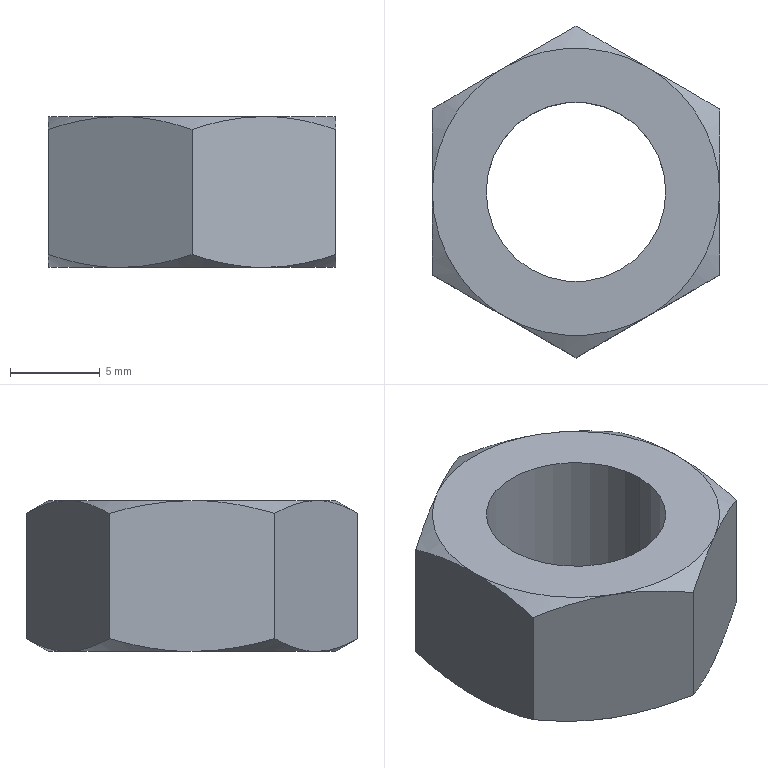Part | SolidWorks | features ICE 3, Extrusion 1, RefAxis 1 | 1 solid | 22 faces | box 16 x 18.475 x 8.4 mm | volume 1194 mm3 | cone 12 | plane 8 | cylinder 2 | commonest cylinder face diameters 10 x2
STEP:
#1=CARTESIAN_POINT('',(-5.,0.,0.));
#2=VERTEX_POINT('',#1);
#3=CARTESIAN_POINT('',(5.,0.,0.));
#4=VERTEX_POINT('',#3);
#5=CARTESIAN_POINT('',(0.,0.,0.));
#6=DIRECTION('',(0.,0.,1.));
#7=DIRECTION('',(1.,0.,0.));
#8=AXIS2_PLACEMENT_3D('',#5,#6,#7);
#9=CIRCLE('',#8,5.);
#10=EDGE_CURVE('',#2,#4,#9,.T.);
#11=ORIENTED_EDGE('',*,*,#10,.F.);
#12=CARTESIAN_POINT('',(-5.,0.,8.4));
#13=VERTEX_POINT('',#12);
#14=CARTESIAN_POINT('',(-5.,0.,0.));
#15=DIRECTION('',(0.,0.,1.));
#16=VECTOR('',#15,1000.);
#17=LINE('',#14,#16);
#18=EDGE_CURVE('',#2,#13,#17,.T.);
#19=ORIENTED_EDGE('',*,*,#18,.T.);
#20=CARTESIAN_POINT('',(5.,0.,8.4));
#21=VERTEX_POINT('',#20);
#22=CARTESIAN_POINT('',(0.,0.,8.4));
#23=DIRECTION('',(0.,0.,1.));
#24=DIRECTION('',(1.,0.,0.));
#25=AXIS2_PLACEMENT_3D('',#22,#23,#24);
#26=CIRCLE('',#25,5.);
#27=EDGE_CURVE('',#13,#21,#26,.T.);
#28=ORIENTED_EDGE('',*,*,#27,.T.);
#29=CARTESIAN_POINT('',(5.,0.,0.));
#30=DIRECTION('',(0.,0.,1.));
#31=VECTOR('',#30,1000.);
#32=LINE('',#29,#31);
#33=EDGE_CURVE('',#4,#21,#32,.T.);
#34=ORIENTED_EDGE('',*,*,#33,.F.);
#35=EDGE_LOOP('',(#11,#19,#28,#34));
#36=FACE_OUTER_BOUND('',#35,.T.);
#37=CARTESIAN_POINT('',(0.,0.,0.));
#38=DIRECTION('',(0.,0.,1.));
#39=DIRECTION('',(1.,0.,0.));
#40=AXIS2_PLACEMENT_3D('',#37,#38,#39);
#41=CYLINDRICAL_SURFACE('',#40,5.);
#42=ADVANCED_FACE('',(#36),#41,.F.);
#43=CARTESIAN_POINT('',(0.,9.238,0.7145));
#44=VERTEX_POINT('',#43);
#45=CARTESIAN_POINT('',(4.,6.928,0.));
#46=VERTEX_POINT('',#45);
#47=CARTESIAN_POINT('',(0.,9.238,0.7145));
#48=CARTESIAN_POINT('',(0.6543,8.86,0.4964));
#49=CARTESIAN_POINT('',(1.313,8.479,0.3167));
#50=CARTESIAN_POINT('',(2.646,7.71,0.0681));
#51=CARTESIAN_POINT('',(3.319,7.322,0.));
#52=CARTESIAN_POINT('',(4.,6.928,0.));
#53=B_SPLINE_CURVE_WITH_KNOTS('',3,(#47,#48,#49,#50,#51,#52),.UNSPECIFIED.,.F.,.F.,(4,2,4),(0.000000238,0.002337,0.004674),.UNSPECIFIED.);
#54=EDGE_CURVE('',#44,#46,#53,.T.);
#55=ORIENTED_EDGE('',*,*,#54,.F.);
#56=CARTESIAN_POINT('',(0.,9.238,7.685));
#57=VERTEX_POINT('',#56);
#58=CARTESIAN_POINT('',(0.,9.238,8.4));
#59=DIRECTION('',(0.,0.,-1.));
#60=VECTOR('',#59,1000.);
#61=LINE('',#58,#60);
#62=EDGE_CURVE('',#57,#44,#61,.T.);
#63=ORIENTED_EDGE('',*,*,#62,.F.);
#64=CARTESIAN_POINT('',(4.,6.928,8.4));
#65=VERTEX_POINT('',#64);
#66=CARTESIAN_POINT('',(4.,6.928,8.4));
#67=CARTESIAN_POINT('',(3.661,7.124,8.4));
#68=CARTESIAN_POINT('',(3.32,7.321,8.383));
#69=CARTESIAN_POINT('',(2.645,7.711,8.318));
#70=CARTESIAN_POINT('',(2.31,7.904,8.269));
#71=CARTESIAN_POINT('',(1.311,8.481,8.083));
#72=CARTESIAN_POINT('',(0.6527,8.861,7.903));
#73=CARTESIAN_POINT('',(0.,9.238,7.685));
#74=B_SPLINE_CURVE_WITH_KNOTS('',3,(#66,#67,#68,#69,#70,#71,#72,#73),.UNSPECIFIED.,.F.,.F.,(4,2,2,4),(0.004674,0.005838,0.007002,0.00933),.UNSPECIFIED.);
#75=EDGE_CURVE('',#65,#57,#74,.T.);
#76=ORIENTED_EDGE('',*,*,#75,.F.);
#77=CARTESIAN_POINT('',(8.,4.619,7.685));
#78=VERTEX_POINT('',#77);
#79=CARTESIAN_POINT('',(8.,4.619,7.685));
#80=CARTESIAN_POINT('',(7.346,4.997,7.904));
#81=CARTESIAN_POINT('',(6.687,5.377,8.083));
#82=CARTESIAN_POINT('',(5.354,6.146,8.332));
#83=CARTESIAN_POINT('',(4.681,6.535,8.4));
#84=CARTESIAN_POINT('',(4.,6.928,8.4));
#85=B_SPLINE_CURVE_WITH_KNOTS('',3,(#79,#80,#81,#82,#83,#84),.UNSPECIFIED.,.F.,.F.,(4,2,4),(0.000000238,0.002337,0.004674),.UNSPECIFIED.);
#86=EDGE_CURVE('',#78,#65,#85,.T.);
#87=ORIENTED_EDGE('',*,*,#86,.F.);
#88=CARTESIAN_POINT('',(8.,4.619,0.7145));
#89=VERTEX_POINT('',#88);
#90=CARTESIAN_POINT('',(8.,4.619,8.4));
#91=DIRECTION('',(0.,0.,-1.));
#92=VECTOR('',#91,1000.);
#93=LINE('',#90,#92);
#94=EDGE_CURVE('',#78,#89,#93,.T.);
#95=ORIENTED_EDGE('',*,*,#94,.T.);
#96=CARTESIAN_POINT('',(4.,6.928,0.));
#97=CARTESIAN_POINT('',(4.339,6.732,0.));
#98=CARTESIAN_POINT('',(4.68,6.535,0.01689));
#99=CARTESIAN_POINT('',(5.355,6.146,0.08225));
#100=CARTESIAN_POINT('',(5.69,5.952,0.1307));
#101=CARTESIAN_POINT('',(6.689,5.376,0.3174));
#102=CARTESIAN_POINT('',(7.347,4.996,0.497));
#103=CARTESIAN_POINT('',(8.,4.619,0.7145));
#104=B_SPLINE_CURVE_WITH_KNOTS('',3,(#96,#97,#98,#99,#100,#101,#102,#103),.UNSPECIFIED.,.F.,.F.,(4,2,2,4),(0.004674,0.005838,0.007002,0.00933),.UNSPECIFIED.);
#105=EDGE_CURVE('',#46,#89,#104,.T.);
#106=ORIENTED_EDGE('',*,*,#105,.F.);
#107=EDGE_LOOP('',(#55,#63,#76,#87,#95,#106));
#108=FACE_OUTER_BOUND('',#107,.T.);
#109=CARTESIAN_POINT('',(8.,4.619,8.4));
#110=DIRECTION('',(-0.5,-0.866,0.));
#111=DIRECTION('',(0.866,-0.5,0.));
#112=AXIS2_PLACEMENT_3D('',#109,#110,#111);
#113=PLANE('',#112);
#114=ADVANCED_FACE('',(#108),#113,.F.);
#115=CARTESIAN_POINT('',(-8.,4.619,0.7145));
#116=VERTEX_POINT('',#115);
#117=CARTESIAN_POINT('',(-4.,6.928,0.));
#118=VERTEX_POINT('',#117);
#119=CARTESIAN_POINT('',(-8.,4.619,0.7145));
#120=CARTESIAN_POINT('',(-7.346,4.997,0.4964));
#121=CARTESIAN_POINT('',(-6.687,5.377,0.3167));
#122=CARTESIAN_POINT('',(-5.354,6.146,0.0681));
#123=CARTESIAN_POINT('',(-4.681,6.535,0.));
#124=CARTESIAN_POINT('',(-4.,6.928,0.));
#125=B_SPLINE_CURVE_WITH_KNOTS('',3,(#119,#120,#121,#122,#123,#124),.UNSPECIFIED.,.F.,.F.,(4,2,4),(0.000000238,0.002337,0.004674),.UNSPECIFIED.);
#126=EDGE_CURVE('',#116,#118,#125,.T.);
#127=ORIENTED_EDGE('',*,*,#126,.F.);
#128=CARTESIAN_POINT('',(-8.,4.619,7.685));
#129=VERTEX_POINT('',#128);
#130=CARTESIAN_POINT('',(-8.,4.619,8.4));
#131=DIRECTION('',(0.,0.,-1.));
#132=VECTOR('',#131,1000.);
#133=LINE('',#130,#132);
#134=EDGE_CURVE('',#129,#116,#133,.T.);
#135=ORIENTED_EDGE('',*,*,#134,.F.);
#136=CARTESIAN_POINT('',(-4.,6.928,8.4));
#137=VERTEX_POINT('',#136);
#138=CARTESIAN_POINT('',(-4.,6.928,8.4));
#139=CARTESIAN_POINT('',(-4.339,6.732,8.4));
#140=CARTESIAN_POINT('',(-4.68,6.535,8.383));
#141=CARTESIAN_POINT('',(-5.355,6.146,8.318));
#142=CARTESIAN_POINT('',(-5.69,5.952,8.269));
#143=CARTESIAN_POINT('',(-6.689,5.376,8.083));
#144=CARTESIAN_POINT('',(-7.347,4.996,7.903));
#145=CARTESIAN_POINT('',(-8.,4.619,7.685));
#146=B_SPLINE_CURVE_WITH_KNOTS('',3,(#138,#139,#140,#141,#142,#143,#144,#145),.UNSPECIFIED.,.F.,.F.,(4,2,2,4),(0.004674,0.005838,0.007002,0.00933),.UNSPECIFIED.);
#147=EDGE_CURVE('',#137,#129,#146,.T.);
#148=ORIENTED_EDGE('',*,*,#147,.F.);
#149=CARTESIAN_POINT('',(0.,9.238,7.685));
#150=CARTESIAN_POINT('',(-0.6543,8.86,7.904));
#151=CARTESIAN_POINT('',(-1.313,8.479,8.083));
#152=CARTESIAN_POINT('',(-2.646,7.71,8.332));
#153=CARTESIAN_POINT('',(-3.319,7.322,8.4));
#154=CARTESIAN_POINT('',(-4.,6.928,8.4));
#155=B_SPLINE_CURVE_WITH_KNOTS('',3,(#149,#150,#151,#152,#153,#154),.UNSPECIFIED.,.F.,.F.,(4,2,4),(0.000000238,0.002337,0.004674),.UNSPECIFIED.);
#156=EDGE_CURVE('',#57,#137,#155,.T.);
#157=ORIENTED_EDGE('',*,*,#156,.F.);
#158=ORIENTED_EDGE('',*,*,#62,.T.);
#159=CARTESIAN_POINT('',(-4.,6.928,0.));
#160=CARTESIAN_POINT('',(-3.661,7.124,0.));
#161=CARTESIAN_POINT('',(-3.32,7.321,0.01689));
#162=CARTESIAN_POINT('',(-2.645,7.711,0.08225));
#163=CARTESIAN_POINT('',(-2.31,7.904,0.1307));
#164=CARTESIAN_POINT('',(-1.311,8.481,0.3174));
#165=CARTESIAN_POINT('',(-0.6527,8.861,0.497));
#166=CARTESIAN_POINT('',(0.,9.238,0.7145));
#167=B_SPLINE_CURVE_WITH_KNOTS('',3,(#159,#160,#161,#162,#163,#164,#165,#166),.UNSPECIFIED.,.F.,.F.,(4,2,2,4),(0.004674,0.005838,0.007002,0.00933),.UNSPECIFIED.);
#168=EDGE_CURVE('',#118,#44,#167,.T.);
#169=ORIENTED_EDGE('',*,*,#168,.F.);
#170=EDGE_LOOP('',(#127,#135,#148,#157,#158,#169));
#171=FACE_OUTER_BOUND('',#170,.T.);
#172=CARTESIAN_POINT('',(0.,9.238,8.4));
#173=DIRECTION('',(0.5,-0.866,0.));
#174=DIRECTION('',(0.866,0.5,0.));
#175=AXIS2_PLACEMENT_3D('',#172,#173,#174);
#176=PLANE('',#175);
#177=ADVANCED_FACE('',(#171),#176,.F.);
#178=CARTESIAN_POINT('',(-8.,-4.619,0.7145));
#179=VERTEX_POINT('',#178);
#180=CARTESIAN_POINT('',(-8.,0.,0.));
#181=VERTEX_POINT('',#180);
#182=CARTESIAN_POINT('',(-8.,-4.619,0.7145));
#183=CARTESIAN_POINT('',(-8.,-3.867,0.4975));
#184=CARTESIAN_POINT('',(-8.,-3.098,0.3157));
#185=CARTESIAN_POINT('',(-8.,-1.557,0.06719));
#186=CARTESIAN_POINT('',(-8.,-0.7811,0.));
#187=CARTESIAN_POINT('',(-8.,0.,0.));
#188=B_SPLINE_CURVE_WITH_KNOTS('',3,(#182,#183,#184,#185,#186,#187),.UNSPECIFIED.,.F.,.F.,(4,2,4),(0.008455,0.01079,0.01313),.UNSPECIFIED.);
#189=EDGE_CURVE('',#179,#181,#188,.T.);
#190=ORIENTED_EDGE('',*,*,#189,.F.);
#191=CARTESIAN_POINT('',(-8.,-4.619,7.685));
#192=VERTEX_POINT('',#191);
#193=CARTESIAN_POINT('',(-8.,-4.619,8.4));
#194=DIRECTION('',(0.,0.,-1.));
#195=VECTOR('',#194,1000.);
#196=LINE('',#193,#195);
#197=EDGE_CURVE('',#192,#179,#196,.T.);
#198=ORIENTED_EDGE('',*,*,#197,.F.);
#199=CARTESIAN_POINT('',(-8.,0.,8.4));
#200=VERTEX_POINT('',#199);
#201=CARTESIAN_POINT('',(-8.,0.,8.4));
#202=CARTESIAN_POINT('',(-8.,-0.7811,8.4));
#203=CARTESIAN_POINT('',(-8.,-1.557,8.333));
#204=CARTESIAN_POINT('',(-8.,-3.098,8.084));
#205=CARTESIAN_POINT('',(-8.,-3.867,7.903));
#206=CARTESIAN_POINT('',(-8.,-4.619,7.685));
#207=B_SPLINE_CURVE_WITH_KNOTS('',3,(#201,#202,#203,#204,#205,#206),.UNSPECIFIED.,.F.,.F.,(4,2,4),(0.03088,0.03322,0.03555),.UNSPECIFIED.);
#208=EDGE_CURVE('',#200,#192,#207,.T.);
#209=ORIENTED_EDGE('',*,*,#208,.F.);
#210=CARTESIAN_POINT('',(-8.,4.619,7.685));
#211=CARTESIAN_POINT('',(-8.,3.872,7.901));
#212=CARTESIAN_POINT('',(-8.,3.115,8.081));
#213=CARTESIAN_POINT('',(-8.,1.574,8.331));
#214=CARTESIAN_POINT('',(-8.,0.7817,8.4));
#215=CARTESIAN_POINT('',(-8.,0.,8.4));
#216=B_SPLINE_CURVE_WITH_KNOTS('',3,(#210,#211,#212,#213,#214,#215),.UNSPECIFIED.,.F.,.F.,(4,2,4),(0.0262,0.02854,0.03088),.UNSPECIFIED.);
#217=EDGE_CURVE('',#129,#200,#216,.T.);
#218=ORIENTED_EDGE('',*,*,#217,.F.);
#219=ORIENTED_EDGE('',*,*,#134,.T.);
#220=CARTESIAN_POINT('',(-8.,0.,0.));
#221=CARTESIAN_POINT('',(-8.,0.7817,0.));
#222=CARTESIAN_POINT('',(-8.,1.574,0.06908));
#223=CARTESIAN_POINT('',(-8.,3.115,0.3194));
#224=CARTESIAN_POINT('',(-8.,3.872,0.4989));
#225=CARTESIAN_POINT('',(-8.,4.619,0.7145));
#226=B_SPLINE_CURVE_WITH_KNOTS('',3,(#220,#221,#222,#223,#224,#225),.UNSPECIFIED.,.F.,.F.,(4,2,4),(0.01313,0.01547,0.01781),.UNSPECIFIED.);
#227=EDGE_CURVE('',#181,#116,#226,.T.);
#228=ORIENTED_EDGE('',*,*,#227,.F.);
#229=EDGE_LOOP('',(#190,#198,#209,#218,#219,#228));
#230=FACE_OUTER_BOUND('',#229,.T.);
#231=CARTESIAN_POINT('',(-8.,4.619,8.4));
#232=DIRECTION('',(1.,0.,0.));
#233=DIRECTION('',(0.,0.,-1.));
#234=AXIS2_PLACEMENT_3D('',#231,#232,#233);
#235=PLANE('',#234);
#236=ADVANCED_FACE('',(#230),#235,.F.);
#237=CARTESIAN_POINT('',(0.,-9.238,0.7145));
#238=VERTEX_POINT('',#237);
#239=CARTESIAN_POINT('',(-4.,-6.928,0.));
#240=VERTEX_POINT('',#239);
#241=CARTESIAN_POINT('',(0.,-9.238,0.7145));
#242=CARTESIAN_POINT('',(-0.6543,-8.86,0.4964));
#243=CARTESIAN_POINT('',(-1.313,-8.479,0.3167));
#244=CARTESIAN_POINT('',(-2.646,-7.71,0.0681));
#245=CARTESIAN_POINT('',(-3.319,-7.322,0.));
#246=CARTESIAN_POINT('',(-4.,-6.928,0.));
#247=B_SPLINE_CURVE_WITH_KNOTS('',3,(#241,#242,#243,#244,#245,#246),.UNSPECIFIED.,.F.,.F.,(4,2,4),(0.000000238,0.002337,0.004674),.UNSPECIFIED.);
#248=EDGE_CURVE('',#238,#240,#247,.T.);
#249=ORIENTED_EDGE('',*,*,#248,.F.);
#250=CARTESIAN_POINT('',(0.,-9.238,7.685));
#251=VERTEX_POINT('',#250);
#252=CARTESIAN_POINT('',(0.,-9.238,8.4));
#253=DIRECTION('',(0.,0.,-1.));
#254=VECTOR('',#253,1000.);
#255=LINE('',#252,#254);
#256=EDGE_CURVE('',#251,#238,#255,.T.);
#257=ORIENTED_EDGE('',*,*,#256,.F.);
#258=CARTESIAN_POINT('',(-4.,-6.928,8.4));
#259=VERTEX_POINT('',#258);
#260=CARTESIAN_POINT('',(-4.,-6.928,8.4));
#261=CARTESIAN_POINT('',(-3.661,-7.124,8.4));
#262=CARTESIAN_POINT('',(-3.32,-7.321,8.383));
#263=CARTESIAN_POINT('',(-2.645,-7.711,8.318));
#264=CARTESIAN_POINT('',(-2.31,-7.904,8.269));
#265=CARTESIAN_POINT('',(-1.311,-8.481,8.083));
#266=CARTESIAN_POINT('',(-0.6527,-8.861,7.903));
#267=CARTESIAN_POINT('',(0.,-9.238,7.685));
#268=B_SPLINE_CURVE_WITH_KNOTS('',3,(#260,#261,#262,#263,#264,#265,#266,#267),.UNSPECIFIED.,.F.,.F.,(4,2,2,4),(0.004674,0.005838,0.007002,0.00933),.UNSPECIFIED.);
#269=EDGE_CURVE('',#259,#251,#268,.T.);
#270=ORIENTED_EDGE('',*,*,#269,.F.);
#271=CARTESIAN_POINT('',(-8.,-4.619,7.685));
#272=CARTESIAN_POINT('',(-7.346,-4.997,7.904));
#273=CARTESIAN_POINT('',(-6.687,-5.377,8.083));
#274=CARTESIAN_POINT('',(-5.354,-6.146,8.332));
#275=CARTESIAN_POINT('',(-4.681,-6.535,8.4));
#276=CARTESIAN_POINT('',(-4.,-6.928,8.4));
#277=B_SPLINE_CURVE_WITH_KNOTS('',3,(#271,#272,#273,#274,#275,#276),.UNSPECIFIED.,.F.,.F.,(4,2,4),(0.000000238,0.002337,0.004674),.UNSPECIFIED.);
#278=EDGE_CURVE('',#192,#259,#277,.T.);
#279=ORIENTED_EDGE('',*,*,#278,.F.);
#280=ORIENTED_EDGE('',*,*,#197,.T.);
#281=CARTESIAN_POINT('',(-4.,-6.928,0.));
#282=CARTESIAN_POINT('',(-4.339,-6.732,0.));
#283=CARTESIAN_POINT('',(-4.68,-6.535,0.01689));
#284=CARTESIAN_POINT('',(-5.355,-6.146,0.08225));
#285=CARTESIAN_POINT('',(-5.69,-5.952,0.1307));
#286=CARTESIAN_POINT('',(-6.689,-5.376,0.3174));
#287=CARTESIAN_POINT('',(-7.347,-4.996,0.497));
#288=CARTESIAN_POINT('',(-8.,-4.619,0.7145));
#289=B_SPLINE_CURVE_WITH_KNOTS('',3,(#281,#282,#283,#284,#285,#286,#287,#288),.UNSPECIFIED.,.F.,.F.,(4,2,2,4),(0.004674,0.005838,0.007002,0.00933),.UNSPECIFIED.);
#290=EDGE_CURVE('',#240,#179,#289,.T.);
#291=ORIENTED_EDGE('',*,*,#290,.F.);
#292=EDGE_LOOP('',(#249,#257,#270,#279,#280,#291));
#293=FACE_OUTER_BOUND('',#292,.T.);
#294=CARTESIAN_POINT('',(-8.,-4.619,8.4));
#295=DIRECTION('',(0.5,0.866,0.));
#296=DIRECTION('',(-0.866,0.5,0.));
#297=AXIS2_PLACEMENT_3D('',#294,#295,#296);
#298=PLANE('',#297);
#299=ADVANCED_FACE('',(#293),#298,.F.);
#300=CARTESIAN_POINT('',(8.,-4.619,0.7145));
#301=VERTEX_POINT('',#300);
#302=CARTESIAN_POINT('',(4.,-6.928,0.));
#303=VERTEX_POINT('',#302);
#304=CARTESIAN_POINT('',(8.,-4.619,0.7145));
#305=CARTESIAN_POINT('',(7.346,-4.997,0.4964));
#306=CARTESIAN_POINT('',(6.687,-5.377,0.3167));
#307=CARTESIAN_POINT('',(5.354,-6.146,0.0681));
#308=CARTESIAN_POINT('',(4.681,-6.535,0.));
#309=CARTESIAN_POINT('',(4.,-6.928,0.));
#310=B_SPLINE_CURVE_WITH_KNOTS('',3,(#304,#305,#306,#307,#308,#309),.UNSPECIFIED.,.F.,.F.,(4,2,4),(0.000000238,0.002337,0.004674),.UNSPECIFIED.);
#311=EDGE_CURVE('',#301,#303,#310,.T.);
#312=ORIENTED_EDGE('',*,*,#311,.F.);
#313=CARTESIAN_POINT('',(8.,-4.619,7.685));
#314=VERTEX_POINT('',#313);
#315=CARTESIAN_POINT('',(8.,-4.619,8.4));
#316=DIRECTION('',(0.,0.,-1.));
#317=VECTOR('',#316,1000.);
#318=LINE('',#315,#317);
#319=EDGE_CURVE('',#314,#301,#318,.T.);
#320=ORIENTED_EDGE('',*,*,#319,.F.);
#321=CARTESIAN_POINT('',(4.,-6.928,8.4));
#322=VERTEX_POINT('',#321);
#323=CARTESIAN_POINT('',(4.,-6.928,8.4));
#324=CARTESIAN_POINT('',(4.339,-6.732,8.4));
#325=CARTESIAN_POINT('',(4.68,-6.535,8.383));
#326=CARTESIAN_POINT('',(5.355,-6.146,8.318));
#327=CARTESIAN_POINT('',(5.69,-5.952,8.269));
#328=CARTESIAN_POINT('',(6.689,-5.376,8.083));
#329=CARTESIAN_POINT('',(7.347,-4.996,7.903));
#330=CARTESIAN_POINT('',(8.,-4.619,7.685));
#331=B_SPLINE_CURVE_WITH_KNOTS('',3,(#323,#324,#325,#326,#327,#328,#329,#330),.UNSPECIFIED.,.F.,.F.,(4,2,2,4),(0.004674,0.005838,0.007002,0.00933),.UNSPECIFIED.);
#332=EDGE_CURVE('',#322,#314,#331,.T.);
#333=ORIENTED_EDGE('',*,*,#332,.F.);
#334=CARTESIAN_POINT('',(0.,-9.238,7.685));
#335=CARTESIAN_POINT('',(0.6543,-8.86,7.904));
#336=CARTESIAN_POINT('',(1.313,-8.479,8.083));
#337=CARTESIAN_POINT('',(2.646,-7.71,8.332));
#338=CARTESIAN_POINT('',(3.319,-7.322,8.4));
#339=CARTESIAN_POINT('',(4.,-6.928,8.4));
#340=B_SPLINE_CURVE_WITH_KNOTS('',3,(#334,#335,#336,#337,#338,#339),.UNSPECIFIED.,.F.,.F.,(4,2,4),(0.000000238,0.002337,0.004674),.UNSPECIFIED.);
#341=EDGE_CURVE('',#251,#322,#340,.T.);
#342=ORIENTED_EDGE('',*,*,#341,.F.);
#343=ORIENTED_EDGE('',*,*,#256,.T.);
#344=CARTESIAN_POINT('',(4.,-6.928,0.));
#345=CARTESIAN_POINT('',(3.661,-7.124,0.));
#346=CARTESIAN_POINT('',(3.32,-7.321,0.01689));
#347=CARTESIAN_POINT('',(2.645,-7.711,0.08225));
#348=CARTESIAN_POINT('',(2.31,-7.904,0.1307));
#349=CARTESIAN_POINT('',(1.311,-8.481,0.3174));
#350=CARTESIAN_POINT('',(0.6527,-8.861,0.497));
#351=CARTESIAN_POINT('',(0.,-9.238,0.7145));
#352=B_SPLINE_CURVE_WITH_KNOTS('',3,(#344,#345,#346,#347,#348,#349,#350,#351),.UNSPECIFIED.,.F.,.F.,(4,2,2,4),(0.004674,0.005838,0.007002,0.00933),.UNSPECIFIED.);
#353=EDGE_CURVE('',#303,#238,#352,.T.);
#354=ORIENTED_EDGE('',*,*,#353,.F.);
#355=EDGE_LOOP('',(#312,#320,#333,#342,#343,#354));
#356=FACE_OUTER_BOUND('',#355,.T.);
#357=CARTESIAN_POINT('',(0.,-9.238,8.4));
#358=DIRECTION('',(-0.5,0.866,0.));
#359=DIRECTION('',(-0.866,-0.5,0.));
#360=AXIS2_PLACEMENT_3D('',#357,#358,#359);
#361=PLANE('',#360);
#362=ADVANCED_FACE('',(#356),#361,.F.);
#363=CARTESIAN_POINT('',(8.,0.,0.));
#364=VERTEX_POINT('',#363);
#365=CARTESIAN_POINT('',(8.,4.619,0.7145));
#366=CARTESIAN_POINT('',(8.,3.872,0.4989));
#367=CARTESIAN_POINT('',(8.,3.115,0.3194));
#368=CARTESIAN_POINT('',(8.,1.574,0.06908));
#369=CARTESIAN_POINT('',(8.,0.7817,0.));
#370=CARTESIAN_POINT('',(8.,0.,0.));
#371=B_SPLINE_CURVE_WITH_KNOTS('',3,(#365,#366,#367,#368,#369,#370),.UNSPECIFIED.,.F.,.F.,(4,2,4),(0.0262,0.02854,0.03088),.UNSPECIFIED.);
#372=EDGE_CURVE('',#89,#364,#371,.T.);
#373=ORIENTED_EDGE('',*,*,#372,.F.);
#374=ORIENTED_EDGE('',*,*,#94,.F.);
#375=CARTESIAN_POINT('',(8.,0.,8.4));
#376=VERTEX_POINT('',#375);
#377=CARTESIAN_POINT('',(8.,0.,8.4));
#378=CARTESIAN_POINT('',(8.,0.7817,8.4));
#379=CARTESIAN_POINT('',(8.,1.574,8.331));
#380=CARTESIAN_POINT('',(8.,3.115,8.081));
#381=CARTESIAN_POINT('',(8.,3.872,7.901));
#382=CARTESIAN_POINT('',(8.,4.619,7.685));
#383=B_SPLINE_CURVE_WITH_KNOTS('',3,(#377,#378,#379,#380,#381,#382),.UNSPECIFIED.,.F.,.F.,(4,2,4),(0.01313,0.01547,0.01781),.UNSPECIFIED.);
#384=EDGE_CURVE('',#376,#78,#383,.T.);
#385=ORIENTED_EDGE('',*,*,#384,.F.);
#386=CARTESIAN_POINT('',(8.,-4.619,7.685));
#387=CARTESIAN_POINT('',(8.,-3.867,7.903));
#388=CARTESIAN_POINT('',(8.,-3.098,8.084));
#389=CARTESIAN_POINT('',(8.,-1.557,8.333));
#390=CARTESIAN_POINT('',(8.,-0.7811,8.4));
#391=CARTESIAN_POINT('',(8.,0.,8.4));
#392=B_SPLINE_CURVE_WITH_KNOTS('',3,(#386,#387,#388,#389,#390,#391),.UNSPECIFIED.,.F.,.F.,(4,2,4),(0.008455,0.01079,0.01313),.UNSPECIFIED.);
#393=EDGE_CURVE('',#314,#376,#392,.T.);
#394=ORIENTED_EDGE('',*,*,#393,.F.);
#395=ORIENTED_EDGE('',*,*,#319,.T.);
#396=CARTESIAN_POINT('',(8.,0.,0.));
#397=CARTESIAN_POINT('',(8.,-0.7811,0.));
#398=CARTESIAN_POINT('',(8.,-1.557,0.06719));
#399=CARTESIAN_POINT('',(8.,-3.098,0.3157));
#400=CARTESIAN_POINT('',(8.,-3.867,0.4975));
#401=CARTESIAN_POINT('',(8.,-4.619,0.7145));
#402=B_SPLINE_CURVE_WITH_KNOTS('',3,(#396,#397,#398,#399,#400,#401),.UNSPECIFIED.,.F.,.F.,(4,2,4),(0.03088,0.03322,0.03555),.UNSPECIFIED.);
#403=EDGE_CURVE('',#364,#301,#402,.T.);
#404=ORIENTED_EDGE('',*,*,#403,.F.);
#405=EDGE_LOOP('',(#373,#374,#385,#394,#395,#404));
#406=FACE_OUTER_BOUND('',#405,.T.);
#407=CARTESIAN_POINT('',(8.,-4.619,8.4));
#408=DIRECTION('',(-1.,0.,0.));
#409=DIRECTION('',(0.,-1.,0.));
#410=AXIS2_PLACEMENT_3D('',#407,#408,#409);
#411=PLANE('',#410);
#412=ADVANCED_FACE('',(#406),#411,.F.);
#413=CARTESIAN_POINT('',(0.,0.,0.));
#414=DIRECTION('',(0.,0.,1.));
#415=DIRECTION('',(1.,0.,0.));
#416=AXIS2_PLACEMENT_3D('',#413,#414,#415);
#417=CIRCLE('',#416,5.);
#418=EDGE_CURVE('',#4,#2,#417,.T.);
#419=ORIENTED_EDGE('',*,*,#418,.T.);
#420=ORIENTED_EDGE('',*,*,#10,.T.);
#421=EDGE_LOOP('',(#419,#420));
#422=FACE_BOUND('',#421,.T.);
#423=CARTESIAN_POINT('',(0.,0.,0.));
#424=DIRECTION('',(0.,0.,1.));
#425=DIRECTION('',(1.,0.,0.));
#426=AXIS2_PLACEMENT_3D('',#423,#424,#425);
#427=CIRCLE('',#426,8.);
#428=EDGE_CURVE('',#364,#46,#427,.T.);
#429=ORIENTED_EDGE('',*,*,#428,.F.);
#430=CARTESIAN_POINT('',(0.,0.,0.));
#431=DIRECTION('',(0.,0.,1.));
#432=DIRECTION('',(1.,0.,0.));
#433=AXIS2_PLACEMENT_3D('',#430,#431,#432);
#434=CIRCLE('',#433,8.);
#435=EDGE_CURVE('',#303,#364,#434,.T.);
#436=ORIENTED_EDGE('',*,*,#435,.F.);
#437=CARTESIAN_POINT('',(0.,0.,0.));
#438=DIRECTION('',(0.,0.,1.));
#439=DIRECTION('',(1.,0.,0.));
#440=AXIS2_PLACEMENT_3D('',#437,#438,#439);
#441=CIRCLE('',#440,8.);
#442=EDGE_CURVE('',#240,#303,#441,.T.);
#443=ORIENTED_EDGE('',*,*,#442,.F.);
#444=CARTESIAN_POINT('',(0.,0.,0.));
#445=DIRECTION('',(0.,0.,1.));
#446=DIRECTION('',(1.,0.,0.));
#447=AXIS2_PLACEMENT_3D('',#444,#445,#446);
#448=CIRCLE('',#447,8.);
#449=EDGE_CURVE('',#181,#240,#448,.T.);
#450=ORIENTED_EDGE('',*,*,#449,.F.);
#451=CARTESIAN_POINT('',(0.,0.,0.));
#452=DIRECTION('',(0.,0.,-1.));
#453=DIRECTION('',(-1.,0.,0.));
#454=AXIS2_PLACEMENT_3D('',#451,#452,#453);
#455=CIRCLE('',#454,8.);
#456=EDGE_CURVE('',#181,#118,#455,.T.);
#457=ORIENTED_EDGE('',*,*,#456,.T.);
#458=CARTESIAN_POINT('',(0.,0.,0.));
#459=DIRECTION('',(0.,0.,1.));
#460=DIRECTION('',(1.,0.,0.));
#461=AXIS2_PLACEMENT_3D('',#458,#459,#460);
#462=CIRCLE('',#461,8.);
#463=EDGE_CURVE('',#46,#118,#462,.T.);
#464=ORIENTED_EDGE('',*,*,#463,.F.);
#465=EDGE_LOOP('',(#429,#436,#443,#450,#457,#464));
#466=FACE_OUTER_BOUND('',#465,.T.);
#467=CARTESIAN_POINT('',(0.,0.,0.));
#468=DIRECTION('',(0.,0.,1.));
#469=DIRECTION('',(1.,0.,0.));
#470=AXIS2_PLACEMENT_3D('',#467,#468,#469);
#471=PLANE('',#470);
#472=ADVANCED_FACE('',(#422,#466),#471,.F.);
#473=CARTESIAN_POINT('',(0.,0.,8.4));
#474=DIRECTION('',(0.,0.,1.));
#475=DIRECTION('',(1.,0.,0.));
#476=AXIS2_PLACEMENT_3D('',#473,#474,#475);
#477=CIRCLE('',#476,5.);
#478=EDGE_CURVE('',#21,#13,#477,.T.);
#479=ORIENTED_EDGE('',*,*,#478,.F.);
#480=ORIENTED_EDGE('',*,*,#27,.F.);
#481=EDGE_LOOP('',(#479,#480));
#482=FACE_BOUND('',#481,.T.);
#483=CARTESIAN_POINT('',(0.,0.,8.4));
#484=DIRECTION('',(0.,0.,1.));
#485=DIRECTION('',(1.,0.,0.));
#486=AXIS2_PLACEMENT_3D('',#483,#484,#485);
#487=CIRCLE('',#486,8.);
#488=EDGE_CURVE('',#322,#376,#487,.T.);
#489=ORIENTED_EDGE('',*,*,#488,.T.);
#490=CARTESIAN_POINT('',(0.,0.,8.4));
#491=DIRECTION('',(0.,0.,1.));
#492=DIRECTION('',(1.,0.,0.));
#493=AXIS2_PLACEMENT_3D('',#490,#491,#492);
#494=CIRCLE('',#493,8.);
#495=EDGE_CURVE('',#376,#65,#494,.T.);
#496=ORIENTED_EDGE('',*,*,#495,.T.);
#497=CARTESIAN_POINT('',(0.,0.,8.4));
#498=DIRECTION('',(0.,0.,1.));
#499=DIRECTION('',(1.,0.,0.));
#500=AXIS2_PLACEMENT_3D('',#497,#498,#499);
#501=CIRCLE('',#500,8.);
#502=EDGE_CURVE('',#65,#137,#501,.T.);
#503=ORIENTED_EDGE('',*,*,#502,.T.);
#504=CARTESIAN_POINT('',(0.,0.,8.4));
#505=DIRECTION('',(0.,0.,1.));
#506=DIRECTION('',(1.,0.,0.));
#507=AXIS2_PLACEMENT_3D('',#504,#505,#506);
#508=CIRCLE('',#507,8.);
#509=EDGE_CURVE('',#137,#200,#508,.T.);
#510=ORIENTED_EDGE('',*,*,#509,.T.);
#511=CARTESIAN_POINT('',(0.,0.,8.4));
#512=DIRECTION('',(0.,0.,1.));
#513=DIRECTION('',(1.,0.,0.));
#514=AXIS2_PLACEMENT_3D('',#511,#512,#513);
#515=CIRCLE('',#514,8.);
#516=EDGE_CURVE('',#200,#259,#515,.T.);
#517=ORIENTED_EDGE('',*,*,#516,.T.);
#518=CARTESIAN_POINT('',(0.,0.,8.4));
#519=DIRECTION('',(0.,0.,1.));
#520=DIRECTION('',(1.,0.,0.));
#521=AXIS2_PLACEMENT_3D('',#518,#519,#520);
#522=CIRCLE('',#521,8.);
#523=EDGE_CURVE('',#259,#322,#522,.T.);
#524=ORIENTED_EDGE('',*,*,#523,.T.);
#525=EDGE_LOOP('',(#489,#496,#503,#510,#517,#524));
#526=FACE_OUTER_BOUND('',#525,.T.);
#527=CARTESIAN_POINT('',(0.,0.,8.4));
#528=DIRECTION('',(0.,0.,1.));
#529=DIRECTION('',(1.,0.,0.));
#530=AXIS2_PLACEMENT_3D('',#527,#528,#529);
#531=PLANE('',#530);
#532=ADVANCED_FACE('',(#482,#526),#531,.T.);
#533=ORIENTED_EDGE('',*,*,#18,.F.);
#534=ORIENTED_EDGE('',*,*,#418,.F.);
#535=ORIENTED_EDGE('',*,*,#33,.T.);
#536=ORIENTED_EDGE('',*,*,#478,.T.);
#537=EDGE_LOOP('',(#533,#534,#535,#536));
#538=FACE_OUTER_BOUND('',#537,.T.);
#539=CARTESIAN_POINT('',(0.,0.,0.));
#540=DIRECTION('',(0.,0.,1.));
#541=DIRECTION('',(1.,0.,0.));
#542=AXIS2_PLACEMENT_3D('',#539,#540,#541);
#543=CYLINDRICAL_SURFACE('',#542,5.);
#544=ADVANCED_FACE('',(#538),#543,.F.);
#545=ORIENTED_EDGE('',*,*,#332,.T.);
#546=ORIENTED_EDGE('',*,*,#393,.T.);
#547=ORIENTED_EDGE('',*,*,#488,.F.);
#548=EDGE_LOOP('',(#545,#546,#547));
#549=FACE_OUTER_BOUND('',#548,.T.);
#550=CARTESIAN_POINT('',(0.,0.,8.4));
#551=DIRECTION('',(0.,0.,-1.));
#552=DIRECTION('',(1.,0.,0.));
#553=AXIS2_PLACEMENT_3D('',#550,#551,#552);
#554=CONICAL_SURFACE('',#553,8.,1.047);
#555=ADVANCED_FACE('',(#549),#554,.T.);
#556=ORIENTED_EDGE('',*,*,#269,.T.);
#557=ORIENTED_EDGE('',*,*,#341,.T.);
#558=ORIENTED_EDGE('',*,*,#523,.F.);
#559=EDGE_LOOP('',(#556,#557,#558));
#560=FACE_OUTER_BOUND('',#559,.T.);
#561=CARTESIAN_POINT('',(0.,0.,8.4));
#562=DIRECTION('',(0.,0.,-1.));
#563=DIRECTION('',(1.,0.,0.));
#564=AXIS2_PLACEMENT_3D('',#561,#562,#563);
#565=CONICAL_SURFACE('',#564,8.,1.047);
#566=ADVANCED_FACE('',(#560),#565,.T.);
#567=ORIENTED_EDGE('',*,*,#208,.T.);
#568=ORIENTED_EDGE('',*,*,#278,.T.);
#569=ORIENTED_EDGE('',*,*,#516,.F.);
#570=EDGE_LOOP('',(#567,#568,#569));
#571=FACE_OUTER_BOUND('',#570,.T.);
#572=CARTESIAN_POINT('',(0.,0.,8.4));
#573=DIRECTION('',(0.,0.,-1.));
#574=DIRECTION('',(1.,0.,0.));
#575=AXIS2_PLACEMENT_3D('',#572,#573,#574);
#576=CONICAL_SURFACE('',#575,8.,1.047);
#577=ADVANCED_FACE('',(#571),#576,.T.);
#578=ORIENTED_EDGE('',*,*,#147,.T.);
#579=ORIENTED_EDGE('',*,*,#217,.T.);
#580=ORIENTED_EDGE('',*,*,#509,.F.);
#581=EDGE_LOOP('',(#578,#579,#580));
#582=FACE_OUTER_BOUND('',#581,.T.);
#583=CARTESIAN_POINT('',(0.,0.,8.4));
#584=DIRECTION('',(0.,0.,-1.));
#585=DIRECTION('',(1.,0.,0.));
#586=AXIS2_PLACEMENT_3D('',#583,#584,#585);
#587=CONICAL_SURFACE('',#586,8.,1.047);
#588=ADVANCED_FACE('',(#582),#587,.T.);
#589=ORIENTED_EDGE('',*,*,#75,.T.);
#590=ORIENTED_EDGE('',*,*,#156,.T.);
#591=ORIENTED_EDGE('',*,*,#502,.F.);
#592=EDGE_LOOP('',(#589,#590,#591));
#593=FACE_OUTER_BOUND('',#592,.T.);
#594=CARTESIAN_POINT('',(0.,0.,8.4));
#595=DIRECTION('',(0.,0.,-1.));
#596=DIRECTION('',(1.,0.,0.));
#597=AXIS2_PLACEMENT_3D('',#594,#595,#596);
#598=CONICAL_SURFACE('',#597,8.,1.047);
#599=ADVANCED_FACE('',(#593),#598,.T.);
#600=ORIENTED_EDGE('',*,*,#86,.T.);
#601=ORIENTED_EDGE('',*,*,#495,.F.);
#602=ORIENTED_EDGE('',*,*,#384,.T.);
#603=EDGE_LOOP('',(#600,#601,#602));
#604=FACE_OUTER_BOUND('',#603,.T.);
#605=CARTESIAN_POINT('',(0.,0.,8.4));
#606=DIRECTION('',(0.,0.,-1.));
#607=DIRECTION('',(1.,0.,0.));
#608=AXIS2_PLACEMENT_3D('',#605,#606,#607);
#609=CONICAL_SURFACE('',#608,8.,1.047);
#610=ADVANCED_FACE('',(#604),#609,.T.);
#611=ORIENTED_EDGE('',*,*,#311,.T.);
#612=ORIENTED_EDGE('',*,*,#435,.T.);
#613=ORIENTED_EDGE('',*,*,#403,.T.);
#614=EDGE_LOOP('',(#611,#612,#613));
#615=FACE_OUTER_BOUND('',#614,.T.);
#616=CARTESIAN_POINT('',(0.,0.,0.));
#617=DIRECTION('',(0.,0.,1.));
#618=DIRECTION('',(-1.,0.,0.));
#619=AXIS2_PLACEMENT_3D('',#616,#617,#618);
#620=CONICAL_SURFACE('',#619,8.,1.047);
#621=ADVANCED_FACE('',(#615),#620,.T.);
#622=ORIENTED_EDGE('',*,*,#248,.T.);
#623=ORIENTED_EDGE('',*,*,#442,.T.);
#624=ORIENTED_EDGE('',*,*,#353,.T.);
#625=EDGE_LOOP('',(#622,#623,#624));
#626=FACE_OUTER_BOUND('',#625,.T.);
#627=CARTESIAN_POINT('',(0.,0.,0.));
#628=DIRECTION('',(0.,0.,1.));
#629=DIRECTION('',(-1.,0.,0.));
#630=AXIS2_PLACEMENT_3D('',#627,#628,#629);
#631=CONICAL_SURFACE('',#630,8.,1.047);
#632=ADVANCED_FACE('',(#626),#631,.T.);
#633=ORIENTED_EDGE('',*,*,#189,.T.);
#634=ORIENTED_EDGE('',*,*,#449,.T.);
#635=ORIENTED_EDGE('',*,*,#290,.T.);
#636=EDGE_LOOP('',(#633,#634,#635));
#637=FACE_OUTER_BOUND('',#636,.T.);
#638=CARTESIAN_POINT('',(0.,0.,0.));
#639=DIRECTION('',(0.,0.,1.));
#640=DIRECTION('',(-1.,0.,0.));
#641=AXIS2_PLACEMENT_3D('',#638,#639,#640);
#642=CONICAL_SURFACE('',#641,8.,1.047);
#643=ADVANCED_FACE('',(#637),#642,.T.);
#644=ORIENTED_EDGE('',*,*,#227,.T.);
#645=ORIENTED_EDGE('',*,*,#126,.T.);
#646=ORIENTED_EDGE('',*,*,#456,.F.);
#647=EDGE_LOOP('',(#644,#645,#646));
#648=FACE_OUTER_BOUND('',#647,.T.);
#649=CARTESIAN_POINT('',(0.,0.,0.));
#650=DIRECTION('',(0.,0.,1.));
#651=DIRECTION('',(-1.,0.,0.));
#652=AXIS2_PLACEMENT_3D('',#649,#650,#651);
#653=CONICAL_SURFACE('',#652,8.,1.047);
#654=ADVANCED_FACE('',(#648),#653,.T.);
#655=ORIENTED_EDGE('',*,*,#168,.T.);
#656=ORIENTED_EDGE('',*,*,#54,.T.);
#657=ORIENTED_EDGE('',*,*,#463,.T.);
#658=EDGE_LOOP('',(#655,#656,#657));
#659=FACE_OUTER_BOUND('',#658,.T.);
#660=CARTESIAN_POINT('',(0.,0.,0.));
#661=DIRECTION('',(0.,0.,1.));
#662=DIRECTION('',(-1.,0.,0.));
#663=AXIS2_PLACEMENT_3D('',#660,#661,#662);
#664=CONICAL_SURFACE('',#663,8.,1.047);
#665=ADVANCED_FACE('',(#659),#664,.T.);
#666=ORIENTED_EDGE('',*,*,#105,.T.);
#667=ORIENTED_EDGE('',*,*,#372,.T.);
#668=ORIENTED_EDGE('',*,*,#428,.T.);
#669=EDGE_LOOP('',(#666,#667,#668));
#670=FACE_OUTER_BOUND('',#669,.T.);
#671=CARTESIAN_POINT('',(0.,0.,0.));
#672=DIRECTION('',(0.,0.,1.));
#673=DIRECTION('',(-1.,0.,0.));
#674=AXIS2_PLACEMENT_3D('',#671,#672,#673);
#675=CONICAL_SURFACE('',#674,8.,1.047);
#676=ADVANCED_FACE('',(#670),#675,.T.);
#677=CLOSED_SHELL('',(#42,#114,#177,#236,#299,#362,#412,#472,#532,#544,#555,#566,#577,#588,#599,#610,#621,#632,#643,#654,#665,#676));
#678=MANIFOLD_SOLID_BREP('',#677);
#679=CARTESIAN_POINT('',(0.,0.,0.));
#680=DIRECTION('',(0.,0.,1.));
#681=DIRECTION('',(1.,0.,0.));
#682=AXIS2_PLACEMENT_3D('',#679,#680,#681);
#683=(LENGTH_UNIT()NAMED_UNIT(*)SI_UNIT(.MILLI.,.METRE.));
#684=UNCERTAINTY_MEASURE_WITH_UNIT(LENGTH_MEASURE(0.00001),#683,'','');
#685=(NAMED_UNIT(*)PLANE_ANGLE_UNIT()SI_UNIT($,.RADIAN.));
#686=(NAMED_UNIT(*)SI_UNIT($,.STERADIAN.)SOLID_ANGLE_UNIT());
#687=(GEOMETRIC_REPRESENTATION_CONTEXT(3)GLOBAL_UNCERTAINTY_ASSIGNED_CONTEXT((#684))GLOBAL_UNIT_ASSIGNED_CONTEXT((#683,#685,#686))REPRESENTATION_CONTEXT('',''));
#688=ADVANCED_BREP_SHAPE_REPRESENTATION('',(#678,#682),#687);